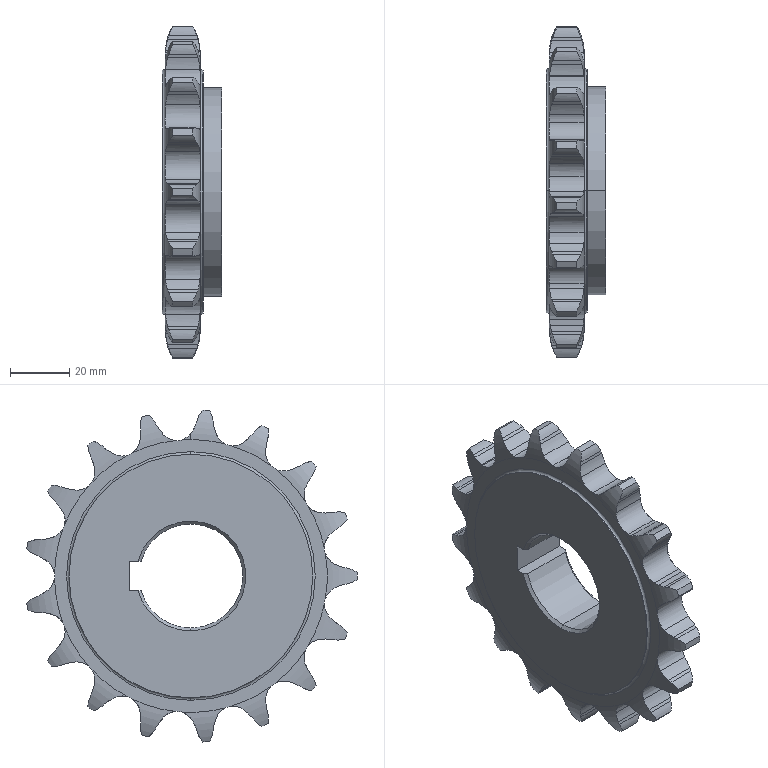Part | SolidWorks | features Chamfer 3, Cut 2, Revolution 2, CirPattern 1, ICE 1 | 1 solid | 207 faces | box 20 x 111.249 x 111.714 mm | volume 104673 mm3 | cylinder 119 | plane 42 | torus 40 | cone 6 | commonest cylinder face diameters 17.45 x36 31.126 x35 12.07 x22 112 x17 82 x4 35 x3